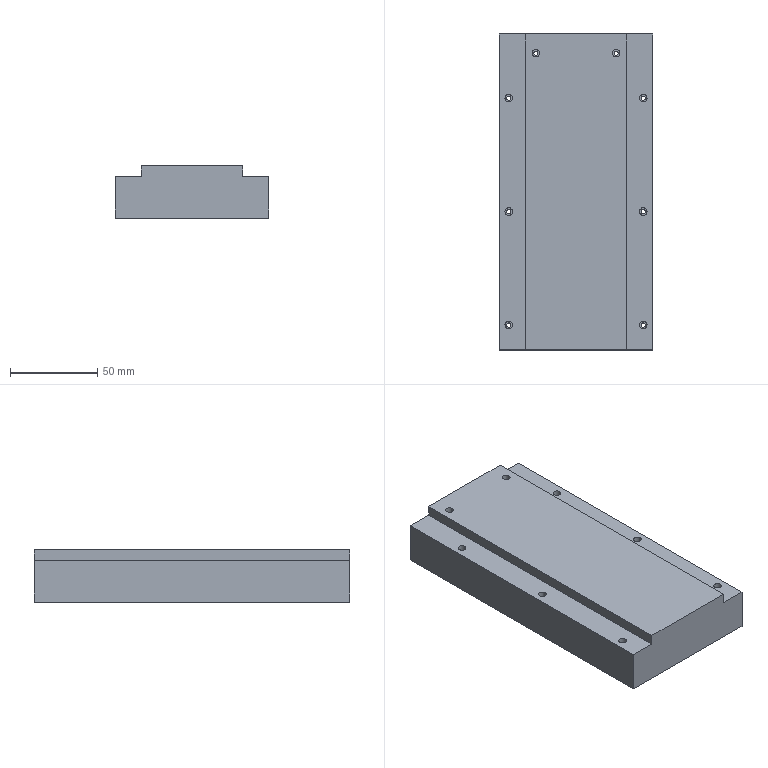NC program | NX | posted with a generic post | part box 88 x 181.05 x 30 mm
Lines 5445 to 6367 of 7800:
(CURVE_DRIVE_1 , TOOL : BALL_END_R1-4-D4-50)
N10870 T14 M6
N10872 G54
N10874 G17 G0 G90 X23.341 Y17.456 B0. C0. S6500 M3
N10876 G43 Z44.5 H14
N10878 Z27.7
N10880 G94 G1 Z25.962 F2000.
N10882 X23.226 Z25.388
N10884 X22.901 Z24.902
N10886 X22.415 Z24.577
N10888 X21.841 Z24.462
N10890 X-21.841
N10892 X-21.891 Y17.21 Z24.406
N10894 X21.891
N10896 X21.942 Y16.963 Z24.35
N10898 X-21.942
N10900 X-21.993 Y16.716 Z24.293
N10902 X21.993
N10904 X22.043 Y16.469 Z24.237
N10906 X-22.043
N10908 X-22.094 Y16.223 Z24.181
N10910 X22.094
N10912 X22.145 Y15.976 Z24.124
N10914 X-22.145
N10916 X-22.196 Y15.729 Z24.068
N10918 X22.196
N10920 X22.246 Y15.483 Z24.012
N10922 X-22.246
N10924 X-22.297 Y15.236 Z23.955
N10926 X22.297
N10928 X22.348 Y14.989 Z23.899
N10930 X-22.348
N10932 X-22.399 Y14.742 Z23.842
N10934 X22.399
N10936 X22.449 Y14.496 Z23.786
N10938 X-22.449
N10940 X-22.5 Y14.249 Z23.73
N10942 X22.5
N10944 X22.551 Y14.002 Z23.673
N10946 X-22.551
N10948 X-22.602 Y13.756 Z23.617
N10950 X22.602
N10952 X23.176 Z23.731
N10954 X23.662 Z24.056
N10956 X23.987 Z24.543
N10958 X24.102 Z25.117
N10960 Z26.5
N10962 G0 Z44.5
(CURVE_DRIVE_1_COPY , TOOL : BALL_END_R1-4-D4-50)
N10964 X23.341 Y17.986
N10966 Z27.7
N10968 G1 Z25.987
N10970 X23.226 Z25.413
N10972 X22.901 Z24.927
N10974 X22.415 Z24.601
N10976 X21.841 Z24.487
N10978 X-21.841
N10980 X-21.876 Y18.288 Z24.447
N10982 X21.876
N10984 X21.912 Y18.589 Z24.408
N10986 X-21.912
N10988 X-21.948 Y18.89 Z24.368
N10990 X21.948
N10992 X21.983 Y19.192 Z24.328
N10994 X-21.983
N10996 X-22.019 Y19.493 Z24.289
N10998 X22.019
N11000 X22.055 Y19.795 Z24.249
N11002 X-22.055
N11004 X-22.091 Y20.096 Z24.209
N11006 X22.091
N11008 X22.126 Y20.398 Z24.17
N11010 X-22.126
N11012 X-22.162 Y20.699 Z24.13
N11014 X22.162
N11016 X22.198 Y21.001 Z24.09
N11018 X-22.198
N11020 X-22.234 Y21.302 Z24.051
N11022 X22.234
N11024 X22.269 Y21.604 Z24.011
N11026 X-22.269
N11028 X-22.305 Y21.905 Z23.971
N11030 X22.305
N11032 X22.341 Y22.207 Z23.932
N11034 X-22.341
N11036 X-22.377 Y22.508 Z23.892
N11038 X22.377
N11040 X22.951 Z24.006
N11042 X23.437 Z24.331
N11044 X23.762 Z24.818
N11046 X23.877 Z25.392
N11048 Z27.1
N11050 G0 Z44.5
(CURVE_DRIVE_1_COPY_1 , TOOL : BALL_END_R1-4-D4-50)
N11052 X31.046 Y84.15
N11054 Z18.7
N11056 G1 Z16.577
N11058 X30.931 Z16.002
N11060 X30.606 Z15.516
N11062 X30.12 Z15.191
N11064 X29.546 Z15.077
N11066 X-29.546
N11068 X-29.823 Y84.294 Z14.768
N11070 X29.823
N11072 X30.101 Y84.437 Z14.46
N11074 X-30.101
N11076 X-30.379 Y84.581 Z14.151
N11078 X30.379
N11080 X30.657 Y84.725 Z13.843
N11082 X-30.657
N11084 X-30.935 Y84.869 Z13.534
N11086 X30.935
N11088 X31.212 Y85.013 Z13.226
N11090 X-31.212
N11092 X-31.49 Y85.157 Z12.917
N11094 X31.49
N11096 X31.768 Y85.301 Z12.609
N11098 X-31.768
N11100 X-32.046 Y85.444 Z12.3
N11102 X32.046
N11104 X32.323 Y85.588 Z11.992
N11106 X-32.323
N11108 X-32.601 Y85.732 Z11.683
N11110 X32.601
N11112 X32.879 Y85.876 Z11.375
N11114 X-32.879
N11116 X-33.157 Y86.02 Z11.066
N11118 X33.157
N11120 X33.434 Y86.164 Z10.758
N11122 X-33.434
N11124 X-33.712 Y86.308 Z10.449
N11126 X33.712
N11128 X34.286 Z10.563
N11130 X34.773 Z10.888
N11132 X35.098 Z11.375
N11134 X35.212 Z11.949
N11136 Z14.5
N11138 G0 Z44.5
(CURVE_DRIVE_2 , TOOL : BALL_END_R1-4-D4-50)
N11140 X-23.035 Y19.774
N11142 Z27.126
N11144 G1 Z25.407 F1000.
N11146 Y19.66 Z24.833
N11148 Y19.335 Z24.346
N11150 Y18.849 Z24.021
N11152 Y18.275 Z23.906
N11154 X-23.036 Y17.576 Z23.911
N11156 X-23.054 Y17.369 Z23.891
N11158 X-23.07 Y17.287 Z23.871
N11160 X-23.069 Y17.696 Z23.874
N11162 Y18.546 Z23.872
N11164 X-23.102 Y18.84 Z23.832
N11166 Y18.688 Z23.837
N11168 X-23.103 Y18.095 Z23.833
N11170 Y17.299 Z23.838
N11172 Y17.113 Z23.83
N11174 X-23.137 Y16.955 Z23.795
N11176 Y17.23 Z23.801
N11178 X-23.136 Y18.293 Z23.796
N11180 Y18.757 Z23.801
N11182 Y19.117 Z23.797
N11184 X-23.169 Y19.388 Z23.763
N11186 X-23.17 Y17.696
N11188 Y16.799 Z23.761
N11190 X-23.204 Y16.642 Z23.727
N11192 X-23.203 Y18.293 Z23.723
N11194 Y19.66 Z23.729
N11196 X-23.236 Y19.944 Z23.692
N11198 X-23.237 Y17.696 Z23.689
N11200 X-23.238 Y16.478 Z23.69
N11202 X-23.271 Y16.311 Z23.651
N11204 X-23.27 Y18.293 Z23.65
N11206 X-23.269 Y20.228 Z23.654
N11208 X-23.302 Y20.524 Z23.614
N11210 X-23.305 Y16.288 Z23.615
N11212 Y16.14 Z23.611
N11214 X-23.338 Y15.97 Z23.571
N11216 Y16.22 Z23.578
N11218 X-23.336 Y20.361 Z23.58
N11220 Y20.812 Z23.576
N11222 X-23.369 Y21.098 Z23.538
N11224 X-23.37 Y19.013 Z23.543
N11226 X-23.372 Y16.151 Z23.541
N11228 Y15.807 Z23.534
N11230 X-23.405 Y15.648 Z23.498
N11232 Y16.8 Z23.504
N11234 X-23.402 Y21.094
N11236 Y21.389 Z23.499
N11238 X-23.436 Y21.66 Z23.465
N11240 X-23.438 Y16.8 Z23.467
N11242 X-23.439 Y15.489 Z23.463
N11244 X-23.472 Y15.328 Z23.427
N11246 X-23.469 Y21.938 Z23.429
N11248 X-23.502 Y22.207 Z23.396
N11250 X-23.506 Y15.165 Z23.39
N11252 X-23.54 Y14.996 Z23.351
N11254 X-23.536 Y22.491 Z23.359
N11256 X-23.569 Y22.786 Z23.319
N11258 X-23.573 Y15.225 Z23.318
N11260 Y14.828 Z23.312
N11262 X-23.607 Y14.662 Z23.274
N11264 X-23.606 Y15.653 Z23.281
N11266 X-23.602 Y22.584 Z23.285
N11268 Y23.081 Z23.279
N11270 X-23.635 Y23.355 Z23.244
N11272 X-23.64 Y15.156 Z23.243
N11274 Y14.503 Z23.238
N11276 X-23.674 Y14.343 Z23.202
N11278 Y14.712 Z23.2
N11280 X-23.673 Y15.593 Z23.206
N11282 X-23.669 Y22.653 Z23.21
N11284 Y23.432 Z23.208
N11286 Y23.658 Z23.202
N11288 X-23.702 Y23.928 Z23.168
N11290 X-23.703 Y21.262 Z23.173
N11292 X-23.706 Y15.088 Z23.169
N11294 X-23.707 Y14.712 Z23.164
N11296 Y14.269 Z23.167
N11298 Y14.172 Z23.161
N11300 X-23.74 Y14.011 Z23.125
N11302 Y14.2 Z23.13
N11304 Y14.712 Z23.127
N11306 X-23.739 Y16.012 Z23.133
N11308 X-23.736 Y22.721 Z23.137
N11310 Y23.067 Z23.132
N11312 X-23.735 Y24.206
N11314 X-23.768 Y24.476 Z23.098
N11316 X-23.773 Y15.019 Z23.095
N11318 X-23.774 Y14.712 Z23.09
N11320 Y13.856 Z23.092
N11322 X-23.808 Y13.694 Z23.055
N11324 X-23.802 Y24.751 Z23.064
N11326 X-23.835 Y25.037 Z23.026
N11328 X-23.841 Y13.529 Z23.018
N11330 X-23.875 Y13.366 Z22.981
N11332 X-23.868 Y25.33 Z22.986
N11334 X-23.902 Y25.615 Z22.949
N11336 X-23.907 Y14.862 Z22.946
N11338 X-23.908 Y13.197 Z22.941
N11340 X-23.941 Y13.03 Z22.902
N11342 Y13.192 Z22.908
N11344 X-23.934 Y25.766 Z22.914
N11346 Y25.9 Z22.91
N11348 X-23.965 Y26.172 Z22.874
N11350 X-23.966 Y24.747 Z22.881
N11352 X-23.972 Y13.128 Z22.873
N11354 Y12.873 Z22.865
N11356 X-24.005 Y12.718 Z22.831
N11358 Y13.589 Z22.838
N11360 X-23.998 Y25.899 Z22.844
N11362 Y26.441 Z22.84
N11364 X-24.031 Y26.726 Z22.802
N11366 X-24.033 Y24.259 Z22.807
N11368 X-24.039 Y12.562 Z22.797
N11370 X-24.072 Y12.405 Z22.763
N11372 X-24.065 Y26.99 Z22.77
N11374 X-24.098 Y27.268 Z22.735
N11376 X-24.106 Y12.238 Z22.724
N11378 X-24.139 Y12.067 Z22.684
N11380 Y12.725 Z22.689
N11382 X-24.131 Y27.56 Z22.695
N11384 X-24.162 Y27.836 Z22.658
N11386 X-24.164 Y25.448 Z22.661
N11388 X-24.171 Y12.224 Z22.654
N11390 Y11.905 Z22.645
N11392 X-24.201 Y11.751 Z22.609
N11394 Y12.193 Z22.62
N11396 X-24.193 Y27.368 Z22.63
N11398 X-24.192 Y28.1 Z22.622
N11400 X-24.222 Y28.375 Z22.584
N11402 Y27.841 Z22.593
N11404 X-24.225 Y22.637 Z22.594
N11406 X-24.231 Y12.163 Z22.587
N11408 Y11.61 Z22.577
N11410 X-24.262 Y11.464 Z22.546
N11412 Y11.728 Z22.542
N11414 Y12.131 Z22.553
N11416 X-24.253 Y28.027 Z22.558
N11418 Y28.438 Z22.549
N11420 Y28.627 Z22.552
N11422 X-24.285 Y28.88 Z22.521
N11424 Y28.438 Z22.514
N11426 X-24.286 Y27.841 Z22.523
N11428 X-24.294 Y12.097 Z22.517
N11430 Y11.728 Z22.507
N11432 Y11.312 Z22.512
N11434 X-24.327 Y11.151 Z22.475
N11436 Y11.728 Z22.472
N11438 Y12.064 Z22.481
N11440 X-24.318 Y28.093 Z22.487
N11442 Y28.438 Z22.479
N11444 Y28.941 Z22.488
N11446 X-24.317 Y29.159 Z22.484
N11448 X-24.351 Y29.423 Z22.452
N11450 Y29.01 Z22.453
N11452 Y28.438 Z22.443
N11454 X-24.352 Y27.841 Z22.45
N11456 X-24.36 Y12.03 Z22.443
N11458 Y11.728 Z22.436
N11460 X-24.361 Y10.994 Z22.441
N11462 X-24.394 Y10.829 Z22.403
N11464 Y11.194 Z22.406
N11466 Y11.728 Z22.399
N11468 Y11.995 Z22.406
N11470 X-24.385 Y28.162 Z22.413
N11472 Y28.438 Z22.407
N11474 X-24.384 Y28.991 Z22.416
N11476 Y29.7 Z22.417
N11478 X-24.417 Y29.986 Z22.378
N11480 X-24.418 Y28.923 Z22.38
N11482 Y28.438 Z22.371
N11484 Y27.599 Z22.379
N11486 X-24.427 Y11.961 Z22.369
N11488 Y11.728 Z22.363
N11490 Y11. Z22.369
N11492 Y10.664 Z22.365
N11494 X-24.46 Y10.503 Z22.328
N11496 Y11.329 Z22.333
N11498 X-24.459 Y11.728 Z22.328
N11500 Y12.419 Z22.334
N11502 X-24.451 Y28.229 Z22.341
N11504 X-24.45 Y28.438 Z22.336
N11506 Y29.333 Z22.344
N11508 X-24.449 Y30.268 Z22.341
N11510 X-24.482 Y30.551 Z22.303
N11512 X-24.483 Y28.789 Z22.307
N11514 Y28.438 Z22.301
N11516 X-24.484 Y26.681 Z22.305
N11518 X-24.492 Y11.894 Z22.297
N11520 Y11.728 Z22.292
N11522 X-24.493 Y10.865 Z22.296
N11524 Y10.344 Z22.292
N11526 X-24.526 Y10.183 Z22.255
N11528 X-24.516 Y28.297 Z22.269
N11530 Y28.438 Z22.265
N11532 Y29.333 Z22.271
N11534 X-24.515 Y30.54 Z22.269
N11536 Y30.845 Z22.263
N11538 X-24.545 Y31.096 Z22.231
N11540 X-24.547 Y28.658 Z22.236
N11542 X-24.557 Y10.138 Z22.223
N11544 Y10.025 Z22.217
N11546 X-24.587 Y9.876 Z22.183
N11548 Y10.076 Z22.19
N11550 X-24.576 Y30.665 Z22.203
N11552 X-24.575 Y31.356 Z22.196
N11554 X-24.607 Y31.618 Z22.163
N11556 X-24.609 Y28.531 Z22.167
N11558 X-24.619 Y10.01 Z22.155
N11560 Y9.728 Z22.151
N11562 X-24.652 Y9.573 Z22.118
N11564 X-24.64 Y31.884 Z22.13
N11566 X-24.674 Y32.163 Z22.094
N11568 X-24.686 Y9.409 Z22.08
N11570 X-24.719 Y9.245 Z22.043
N11572 X-24.707 Y32.452 Z22.056
N11574 X-24.739 Y32.733 Z22.019
N11576 X-24.752 Y9.082 Z22.005
N11578 X-24.783 Y8.924 Z21.968
N11580 Y9.341 Z21.973
N11582 X-24.77 Y32.735 Z21.985
N11584 Y33.014 Z21.98
N11586 X-24.799 Y33.269 Z21.945
N11588 Y32.168 Z21.956
N11590 X-24.812 Y9.017 Z21.941
N11592 Y8.775 Z21.932
N11594 X-24.842 Y8.633 Z21.901
N11596 X-24.841 Y8.956 Z21.908
N11598 X-24.829 Y32.795 Z21.921
N11600 X-24.828 Y33.212 Z21.912
N11602 Y33.503 Z21.916
N11604 X-24.859 Y33.771 Z21.88
N11606 Y33.633 Z21.885
N11608 Y33.212 Z21.879
N11610 Y32.616 Z21.887
N11612 X-24.872 Y8.893 Z21.874
N11614 Y8.488 Z21.869
N11616 X-24.905 Y8.337 Z21.836
N11618 X-24.891 Y32.859 Z21.851
N11620 Y33.212 Z21.844
N11622 Y33.699 Z21.851
N11624 Y34.031 Z21.847
N11626 X-24.924 Y34.296 Z21.815
N11628 Y33.767 Z21.816
N11630 X-24.925 Y33.212 Z21.808
N11632 Y32.297 Z21.816
N11634 X-24.938 Y8.18 Z21.801
N11636 X-24.971 Y8.018 Z21.764
N11638 X-24.957 Y32.927 Z21.778
N11640 Y33.212 Z21.773
N11642 Y33.784 Z21.781
N11644 X-24.956 Y34.565 Z21.78
N11646 X-24.989 Y34.846 Z21.743
N11648 X-24.99 Y33.717 Z21.744
N11650 Y33.212 Z21.737
N11652 Y32.364 Z21.743
N11654 X-25.004 Y7.853 Z21.725
N11656 X-25.036 Y7.692 Z21.688
N11658 X-25.035 Y7.961 Z21.693
N11660 X-25.022 Y32.993 Z21.707
N11662 Y33.212 Z21.703
N11664 X-25.021 Y34.107 Z21.709
N11666 Y35.117 Z21.708
N11668 X-25.052 Y35.392 Z21.67
N11670 X-25.053 Y33.587 Z21.674
N11672 Y33.212 Z21.669
N11674 X-25.054 Y30.27 Z21.672
N11676 X-25.066 Y7.897 Z21.659
N11678 X-25.067 Y7.537 Z21.652
N11680 X-25.098 Y7.386 Z21.618
N11682 Y7.833 Z21.624
N11684 X-25.084 Y33.058 Z21.638
N11686 X-25.083 Y35.287 Z21.639
N11688 Y35.668 Z21.633
N11690 X-25.115 Y35.932 Z21.599
N11692 X-25.116 Y33.457 Z21.604
N11694 X-25.13 Y7.767 Z21.588
N11696 Y7.233 Z21.584
N11698 X-25.163 Y7.073 Z21.547
N11700 X-25.162 Y9.252 Z21.553
N11702 X-25.148 Y35.42 Z21.568
N11704 X-25.147 Y36.224 Z21.559
N11706 X-25.178 Y36.474 Z21.528
N11708 X-25.18 Y34.107 Z21.533
N11710 X-25.194 Y7.038 Z21.515
N11712 Y6.915 Z21.51
N11714 X-25.228 Y6.761 Z21.477
N11716 X-25.212 Y36.741 Z21.495
N11718 X-25.245 Y37.016 Z21.46
N11720 X-25.261 Y6.598 Z21.44
N11722 X-25.295 Y6.432 Z21.402
N11724 X-25.278 Y37.301 Z21.423
N11726 X-25.31 Y37.587 Z21.384
N11728 X-25.327 Y6.86 Z21.37
N11730 Y6.273 Z21.366
N11732 X-25.36 Y6.115 Z21.33
N11734 X-25.343 Y37.501 Z21.35
N11736 Y37.882 Z21.343
N11738 X-25.375 Y38.152 Z21.308
N11740 X-25.376 Y36.466 Z21.315
N11742 X-25.392 Y6.034 Z21.295
N11744 Y5.95 Z21.291
N11746 X-25.423 Y5.792 Z21.253
N11748 Y5.972 Z21.262
N11750 X-25.406 Y37.565 Z21.281
N11752 Y37.987 Z21.273
N11754 X-25.405 Y38.407 Z21.275
N11756 X-25.436 Y38.675 Z21.239
N11758 Y38.399 Z21.245
N11760 Y37.987 Z21.24
N11762 X-25.437 Y37. Z21.248
N11764 X-25.453 Y5.909 Z21.228
N11766 X-25.454 Y5.647 Z21.221
N11768 X-25.486 Y5.494 Z21.188
N11770 X-25.484 Y10.963 Z21.196
N11772 X-25.469 Y37.63 Z21.21
N11774 Y37.987 Z21.204
N11776 Y38.466 Z21.21
N11778 Y38.938 Z21.206
N11780 X-25.502 Y39.215 Z21.171
N11782 Y38.535 Z21.174
N11784 Y37.987 Z21.168
N11786 X-25.503 Y37.068 Z21.174
N11788 X-25.52 Y5.339 Z21.154
N11790 X-25.554 Y5.176 Z21.117
N11792 X-25.536 Y37.699 Z21.136
N11794 Y37.987 Z21.131
N11796 X-25.535 Y39.161 Z21.138
N11798 Y39.482
N11800 X-25.568 Y39.767 Z21.1
N11802 X-25.569 Y38.495 Z21.101
N11804 Y37.987 Z21.095
N11806 X-25.57 Y36.659 Z21.1
N11808 X-25.587 Y5.011 Z21.079
N11810 X-25.621 Y4.839 Z21.039
N11812 X-25.62 Y5.953 Z21.044
N11814 X-25.603 Y37.767 Z21.062
N11816 Y37.987 Z21.059
N11818 X-25.602 Y39.18 Z21.064
N11820 Y40.058 Z21.061
N11822 X-25.634 Y40.343 Z21.023
N11824 Y39.403 Z21.028
N11826 X-25.635 Y37.39 Z21.027
N11828 X-25.653 Y4.903 Z21.007
N11830 Y4.675 Z21.
N11832 X-25.684 Y4.52 Z20.964
N11834 Y4.839 Z20.973
N11836 X-25.665 Y40.062 Z20.994
N11838 Y40.604 Z20.989
N11840 X-25.697 Y40.891 Z20.949
N11842 Y39.777 Z20.958
N11844 X-25.716 Y4.773 Z20.937
N11846 Y4.367 Z20.93
N11848 X-25.75 Y4.209 Z20.895
N11850 X-25.748 Y7.384 Z20.902
N11852 X-25.73 Y40.793 Z20.918
N11854 Y41.17 Z20.913
N11856 X-25.763 Y41.439 Z20.88
N11858 X-25.766 Y36.893 Z20.882
N11860 X-25.783 Y4.051 Z20.86
N11862 X-25.817 Y3.891 Z20.824
N11864 X-25.797 Y41.716 Z20.844
N11866 X-25.83 Y41.987 Z20.81
N11868 X-25.85 Y3.72 Z20.785
N11870 X-25.884 Y3.551 Z20.745
N11872 Y4.489 Z20.752
N11874 X-25.863 Y42.274 Z20.772
N11876 X-25.896 Y42.564 Z20.733
N11878 Y40.978 Z20.737
N11880 X-25.916 Y3.867 Z20.715
N11882 X-25.917 Y3.387 Z20.707
N11884 X-25.949 Y3.233 Z20.672
N11886 X-25.948 Y4.424 Z20.68
N11888 X-25.928 Y42.279 Z20.701
N11890 Y42.844 Z20.695
N11892 X-25.961 Y43.123 Z20.659
N11894 X-25.962 Y40.977 Z20.665
N11896 X-25.982 Y3.8 Z20.642
N11898 Y3.373 Z20.635
N11900 Y3.075 Z20.637
N11902 X-26.016 Y2.908 Z20.598
N11904 X-26.015 Y4.934 Z20.606
N11906 X-25.995 Y42.347 Z20.628
N11908 X-25.994 Y42.761 Z20.622
N11910 Y43.125 Z20.625
N11912 Y43.42 Z20.619
N11914 X-26.026 Y43.679 Z20.586
N11916 Y43.191 Z20.59
N11918 Y42.761 Z20.587
N11920 X-26.027 Y41.783 Z20.592
N11922 X-26.047 Y3.733 Z20.57
N11924 X-26.048 Y3.373 Z20.563
N11926 Y2.898 Z20.567
N11928 Y2.745 Z20.56
N11930 X-26.081 Y2.591 Z20.527
N11932 Y2.83 Z20.531
N11934 Y3.373 Z20.527
N11936 X-26.08 Y4.281 Z20.533
N11938 X-26.06 Y42.414 Z20.555
N11940 Y42.761 Z20.55
N11942 X-26.059 Y43.856 Z20.552
N11944 Y43.964 Z20.548
N11946 X-26.092 Y44.225 Z20.517
N11948 X-26.093 Y42.761 Z20.514
N11950 X-26.094 Y41.554 Z20.518
N11952 X-26.114 Y3.664 Z20.495
N11954 Y3.373 Z20.49
N11956 X-26.115 Y2.435 Z20.493
N11958 X-26.148 Y2.27 Z20.455
N11960 Y3.373 Z20.454
N11962 X-26.147 Y5.324 Z20.459
N11964 X-26.127 Y42.483 Z20.481
N11966 Y42.761 Z20.477
N11968 X-26.126 Y44.498 Z20.482
N11970 X-26.159 Y44.787 Z20.444
N11972 X-26.182 Y2.106 Z20.418
N11974 X-26.215 Y1.943 Z20.38
N11976 X-26.192 Y44.705 Z20.408
N11978 Y45.082 Z20.404
N11980 X-26.225 Y45.364 Z20.367
N11982 X-26.227 Y43.113 Z20.371
N11984 X-26.249 Y1.889 Z20.344
N11986 Y1.77 Z20.339
N11988 X-26.281 Y1.605 Z20.3
N11990 Y1.824 Z20.309
N11992 X-26.257 Y44.846 Z20.336
N11994 Y45.651 Z20.327
N11996 X-26.289 Y45.923 Z20.292
N11998 X-26.29 Y44.431 Z20.3
N12000 X-26.313 Y1.757 Z20.274
N12002 Y1.452 Z20.266
N12004 X-26.347 Y1.296 Z20.232
N12006 X-26.345 Y3.265 Z20.238
N12008 X-26.323 Y45.591 Z20.262
N12010 X-26.322 Y46.195 Z20.257
N12012 X-26.356 Y46.479 Z20.22
N12014 X-26.357 Y43.951 Z20.226
N12016 X-26.38 Y1.14 Z20.198
N12018 X-26.413 Y0.98 Z20.162
N12020 X-26.389 Y46.74 Z20.189
N12022 X-26.422 Y47.016 Z20.153
N12024 X-26.447 Y0.814 Z20.124
N12026 X-26.478 Y0.655 Z20.087
N12028 Y0.984 Z20.09
N12030 X-26.453 Y47.29 Z20.116
N12032 X-26.484 Y47.563 Z20.08
N12034 X-26.485 Y46.197 Z20.082
N12036 X-26.509 Y0.757 Z20.056
N12038 Y0.496 Z20.049
N12040 X-26.543 Y0.331 Z20.011
N12042 X-26.542 Y0.689 Z20.02
N12044 X-26.517 Y47.184 Z20.047
N12046 Y47.847 Z20.042
N12048 X-26.549 Y48.138 Z20.002
N12050 Y47.846 Z20.009
N12052 X-26.575 Y0.623 Z19.984
N12054 Y0.179 Z19.977
N12056 X-26.608 Y0.021 Z19.942
N12058 Y0.555 Z19.947
N12060 X-26.602 Y10.314 Z19.949
N12062 X-26.582 Y47.914 Z19.973
N12064 Y48.408 Z19.968
N12066 X-26.615 Y48.695 Z19.929
N12068 X-26.616 Y47.386 Z19.938
N12070 X-26.618 Y42.628 Z19.931
N12072 X-26.641 Y0.954 Z19.906
N12074 Y-0.11 Z19.907
N12076 Y-0.141 Z19.905
N12078 X-26.674 Y-0.301 Z19.869
N12080 Y0.419 Z19.874
N12082 X-26.673 Y2.394 Z19.87
N12084 X-26.649 Y46.921 Z19.897
N12086 X-26.648 Y48.05 Z19.901
N12088 Y48.96 Z19.896
N12090 X-26.681 Y49.22 Z19.865
N12092 X-26.682 Y47.521
N12094 Y46.2 Z19.859
N12096 X-26.707 Y0.961 Z19.832
N12098 Y-0.262 Z19.836
N12100 X-26.708 Y-0.462 Z19.833
N12102 X-26.74 Y-0.629 Z19.794
N12104 Y0.494 Z19.799
N12106 X-26.738 Y3.837 Z19.796
N12108 X-26.715 Y46.939 Z19.822
N12110 X-26.714 Y48.888 Z19.828
N12112 Y49.502 Z19.827
N12114 X-26.746 Y49.794 Z19.788
N12116 X-26.748 Y47.414 Z19.79
N12118 X-26.749 Y44.065 Z19.783
N12120 X-26.773 Y-0.381 Z19.76
N12122 Y-0.729 Z19.756
N12124 X-26.805 Y-0.746 Z19.72
N12126 X-26.804 Y0.625 Z19.725
N12128 X-26.779 Y46.939 Z19.75
N12130 X-26.777 Y49.836 Z19.752
N12132 X-26.809 Y49.717 Z19.718
N12134 X-26.836 Y-0.763 Z19.685
N12136 X-26.867 Y-0.78 Z19.65
N12138 X-26.84 Y49.598 Z19.684
N12140 X-26.839 Y50.172 Z19.798
N12142 Y50.658 Z20.124
N12144 Y50.983 Z20.611
N12146 Y51.097 Z21.185
N12148 Z22.979
N12150 G0 Z44.5
N12152 X23.035 Y16.086
N12154 Z27.071
N12156 G1 Z25.417
N12158 Y16.198 Z24.843
N12160 Y16.522 Z24.355
N12162 Y17.007 Z24.028
N12164 Y17.581 Z23.912
N12166 Y18.276 Z23.906
N12168 X23.069 Y18.549 Z23.872
N12170 Y17.291
N12172 X23.102 Y17.118 Z23.831
N12174 Y17.3 Z23.839
N12176 Y18.293 Z23.833
N12178 Y18.688 Z23.837
N12180 Y18.845 Z23.832
N12182 X23.135 Y19.113 Z23.798
N12184 Y18.755 Z23.802
N12186 Y18.061 Z23.798
N12188 Y17.233 Z23.803
N12190 Y16.965 Z23.797
N12192 X23.168 Y16.809 Z23.763
N12194 Y17.696 Z23.765
N12196 Y18.293 Z23.761
N12198 Y19.385 Z23.764
N12200 X23.202 Y19.659 Z23.729
N12202 Y17.993 Z23.724
N12204 Y16.653 Z23.729
N12206 X23.235 Y16.489 Z23.692
N12208 Y18.293 Z23.688
N12210 Y19.944 Z23.692
N12212 X23.269 Y20.229 Z23.655
N12214 Y17.696 Z23.654
N12216 Y16.324
N12218 X23.302 Y16.153 Z23.614
N12220 Y17.308 Z23.618
N12222 Y20.527 Z23.614
N12224 X23.336 Y20.816 Z23.576
N12226 Y18.611 Z23.581
N12228 Y16.224
N12230 Y15.983 Z23.574
N12232 X23.369 Y15.822 Z23.537
N12234 Y16.157 Z23.544
N12236 Y21.025 Z23.541
N12238 Y21.098 Z23.539
N12240 X23.402 Y21.39 Z23.499
N12242 Y19.992 Z23.507
N12244 Y16.088
N12246 Y15.664 Z23.502
N12248 X23.436 Y15.506 Z23.467
N12250 Y21.163 Z23.468
N12252 Y21.662 Z23.465
N12254 X23.469 Y21.941 Z23.429
N12256 Y15.346 Z23.431
N12258 X23.503 Y15.183 Z23.394
N12260 Y22.212 Z23.396
N12262 X23.536 Y22.497 Z23.358
N12264 Y15.015 Z23.355
N12266 X23.569 Y14.847 Z23.316
N12268 Y15.228 Z23.322
N12270 Y22.794 Z23.318
N12272 X23.603 Y23.09 Z23.278
N12274 Y22.123 Z23.284
N12276 Y15.194
N12278 Y14.681 Z23.278
N12280 X23.636 Y14.522 Z23.242
N12282 Y16.558 Z23.247
N12284 Y22.619
N12286 Y23.364 Z23.243
N12288 X23.67 Y23.67 Z23.201
N12290 Y23.434 Z23.207
N12292 Y23.067 Z23.205
N12294 Y21.713 Z23.21
N12296 Y15.125
N12298 Y14.712 Z23.204
N12300 Y14.363 Z23.207
N12302 X23.703 Y14.192 Z23.166
N12304 Y14.276 Z23.171
N12306 Y14.712 Z23.167
N12308 Y15.566 Z23.173
N12310 Y22.688
N12312 Y23.067 Z23.168
N12314 Y23.502 Z23.171
N12316 Y23.943 Z23.166
N12318 X23.737 Y24.224 Z23.13
N12320 Y23.571 Z23.135
N12322 Y23.067 Z23.131
N12324 Y20.806 Z23.136
N12326 Y15.057
N12328 Y14.712 Z23.131
N12330 Y14.208 Z23.134
N12332 Y14.029 Z23.129
N12334 X23.77 Y13.875 Z23.096
N12336 Y14.712 Z23.094
N12338 Y15.989 Z23.099
N12340 Y23.067 Z23.094
N12342 Y24.493 Z23.097
N12344 X23.804 Y24.77 Z23.061
N12346 Y14.988
N12348 Y14.454 Z23.059
N12350 Y13.714 Z23.06
N12352 X23.837 Y13.55 Z23.022
N12354 Y25.058 Z23.023
N12356 X23.871 Y25.353 Z22.984
N12358 Y13.387 Z22.985
N12360 X23.904 Y13.22 Z22.947
N12362 Y25.108 Z22.95
N12364 Y25.638 Z22.946
N12366 X23.937 Y25.936 Z22.906
N12368 Y24.719 Z22.913
N12370 Y13.199 Z22.912
N12372 Y13.048 Z22.906
N12374 X23.971 Y12.881 Z22.867
N12376 Y13.13 Z22.875
N12378 Y25.842 Z22.874
N12380 Y26.22 Z22.868
N12382 X24.004 Y26.493 Z22.834
N12384 Y22.483 Z22.839
N12386 Y13.062 Z22.838
N12388 Y12.725 Z22.832
N12390 X24.038 Y12.568 Z22.798
N12392 Y26.576 Z22.799
N12394 Y26.778 Z22.796
N12396 X24.071 Y27.042 Z22.764
N12398 Y12.412
N12400 X24.105 Y12.246 Z22.726
N12402 Y27.328 Z22.727
N12404 X24.138 Y27.623 Z22.687
N12406 Y12.257 Z22.69
N12408 Y12.075 Z22.685
N12410 X24.171 Y11.903 Z22.645
N12412 Y12.223 Z22.653
N12414 Y27.346
N12416 Y27.914 Z22.648
N12418 X24.204 Y28.215 Z22.607
N12420 Y27.38 Z22.617
N12422 Y12.189 Z22.616
N12424 Y11.735 Z22.605
N12426 X24.238 Y11.578 Z22.57
N12428 Y11.728 Z22.568
N12430 Y12.155 Z22.579
N12432 Y27.414
N12434 Y28.011 Z22.575
N12436 Y28.512 Z22.566
N12438 X24.271 Y28.773 Z22.535
N12440 Y28.438 Z22.529
N12442 Y27.841 Z22.539
N12444 Y12.121 Z22.542
N12446 Y11.728 Z22.532
N12448 Y11.422 Z22.536
N12450 X24.305 Y11.265 Z22.502
N12452 Y11.728 Z22.496
N12454 Y12.086 Z22.505
N12456 Y28.08 Z22.502
N12458 Y28.438 Z22.493
N12460 Y28.915 Z22.501
N12462 Y29.059 Z22.497
N12464 X24.338 Y29.325 Z22.464
N12466 Y28.983 Z22.466
N12468 Y28.438 Z22.457
N12470 Y27.841 Z22.465
N12472 Y12.052 Z22.468
N12474 Y11.728 Z22.46
N12476 Y11.131 Z22.463
N12478 Y11.099
N12480 X24.372 Y10.942 Z22.429
N12482 Y11.728 Z22.423
N12484 Y12.018 Z22.431
N12486 Y28.148 Z22.428
N12488 Y28.438 Z22.421
N12490 Y29.035 Z22.431
N12492 Y29.595
N12494 X24.405 Y29.884 Z22.392
N12496 Y28.949 Z22.394
N12498 Y28.438 Z22.385
N12500 Y27.586 Z22.394
N12502 Y11.983
N12504 Y11.728 Z22.387
N12506 Y11.045 Z22.394
N12508 Y10.776 Z22.391
N12510 X24.438 Y10.61 Z22.352
N12512 Y11.286 Z22.356
N12514 Y11.728 Z22.351
N12516 Y11.949 Z22.356
N12518 Y28.217 Z22.354
N12520 Y28.438 Z22.349
N12522 Y29.333 Z22.356
N12524 Y30.175 Z22.354
N12526 X24.472 Y30.46 Z22.316
N12528 Y28.812 Z22.319
N12530 Y28.438 Z22.313
N12532 Y27.163 Z22.319
N12534 Y11.915
N12536 Y11.728 Z22.315
N12538 Y10.908 Z22.319
N12540 Y10.446 Z22.315
N12542 X24.505 Y10.285 Z22.279
N12544 Y11.423 Z22.282
N12546 Y11.728 Z22.278
N12548 Y16.326 Z22.282
N12550 Y28.286 Z22.281
N12552 Y28.438 Z22.277
N12554 Y29.333 Z22.282
N12556 Y30.52 Z22.28
N12558 Y30.764 Z22.274
N12560 X24.539 Y31.045 Z22.238
N12562 Y29.333 Z22.245
N12564 Y27.841 Z22.244
N12566 Y10.174 Z22.242
N12568 Y10.117 Z22.239
N12570 X24.572 Y9.944 Z22.198
N12572 Y10.105 Z22.206
N12574 Y30.658 Z22.207
N12576 Y31.331 Z22.2
N12578 X24.606 Y31.61 Z22.164
N12580 Y29.333 Z22.171
N12582 Y10.036 Z22.17
N12584 Y9.789 Z22.164
N12586 X24.639 Y9.634 Z22.131
N12588 Y31.877 Z22.132
N12590 X24.673 Y32.156 Z22.096
N12592 Y9.474 Z22.095
N12594 X24.706 Y9.31 Z22.058
N12596 Y32.447 Z22.057
N12598 X24.74 Y32.737 Z22.018
N12600 Y9.146 Z22.02
N12602 X24.773 Y8.975 Z21.98
N12604 Y9.937 Z21.985
N12606 Y32.738 Z21.982
N12608 Y33.044 Z21.976
N12610 X24.806 Y33.333 Z21.938
N12612 Y32.175 Z21.948
N12614 Y9.027 Z21.947
N12616 Y8.803 Z21.939
N12618 X24.839 Y8.646 Z21.903
N12620 Y8.961 Z21.911
N12622 Y32.805 Z21.909
N12624 Y33.212 Z21.901
N12626 Y33.589 Z21.906
N12628 X24.872 Y33.885 Z21.866
N12630 Y33.661 Z21.871
N12632 Y33.212 Z21.865
N12634 Y32.616 Z21.872
N12636 Y8.892 Z21.874
N12638 Y8.489 Z21.869
N12640 X24.906 Y8.332 Z21.834
N12642 Y32.874 Z21.835
N12644 Y33.212 Z21.828
N12646 Y33.809 Z21.833
N12648 Y34.153
N12650 X24.939 Y34.423 Z21.799
N12652 Y33.798 Z21.8
N12654 Y33.212 Z21.792
N12656 Y32.312 Z21.8
N12658 Y8.175
N12660 X24.973 Y8.009 Z21.762
N12662 Y32.943
N12664 Y33.212 Z21.756
N12666 Y33.752 Z21.763
N12668 Y34.706 Z21.762
N12670 X25.006 Y34.991 Z21.724
N12672 Y33.684 Z21.727
N12674 Y33.212 Z21.72
N12676 Y32.38 Z21.727
N12678 Y7.843 Z21.723
N12680 X25.038 Y7.682 Z21.685
N12682 Y8.445 Z21.691
N12684 Y33.01 Z21.69
N12686 Y33.212 Z21.686
N12688 Y34.128 Z21.691
N12690 Y35.268 Z21.688